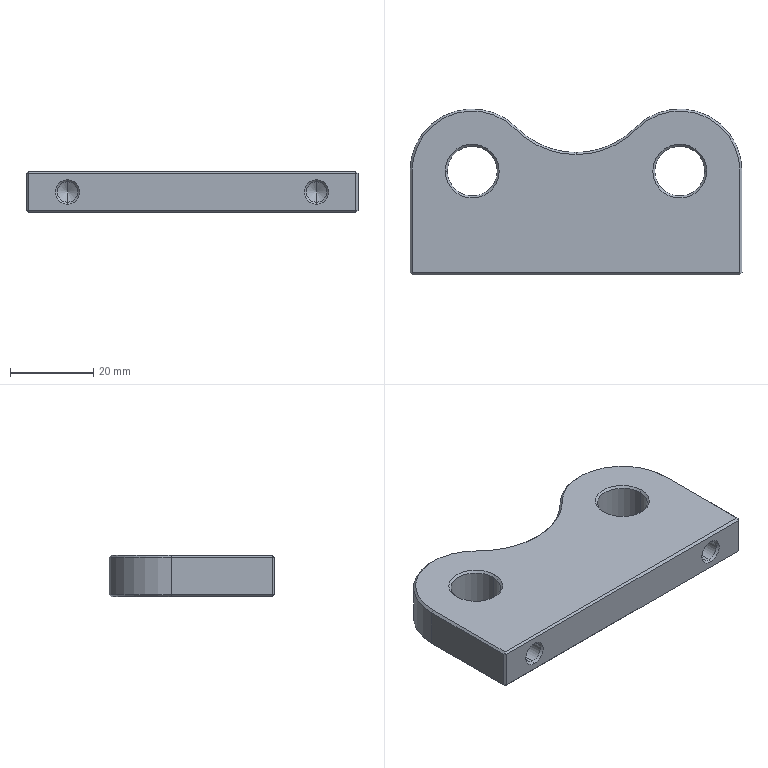Part | STEP file | Roll shaft support seat | 1 solid | 51 faces | box 80 x 40 x 10 mm | volume 25332 mm3 | cone 23 | plane 17 | cylinder 11 | commonest cylinder face diameters 4.917 x4 12 x4 30 x2 40 x1